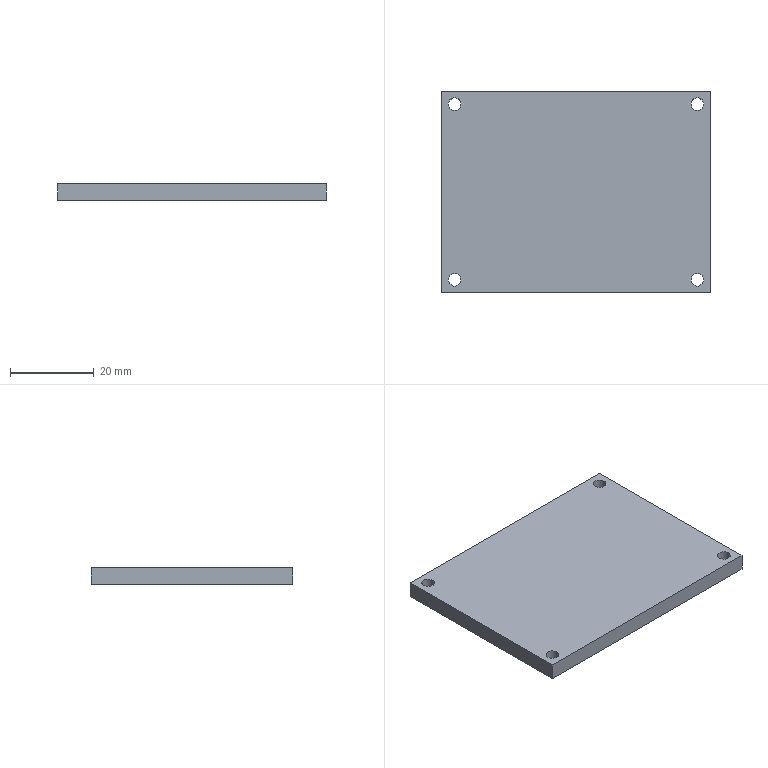Part | SolidWorks | features Extrusion 1, ICE 1 | 1 solid | 14 faces | box 64 x 48 x 4 mm | volume 12175 mm3 | cylinder 8 | plane 6 | commonest cylinder face diameters 3 x8
STEP:
#1=CARTESIAN_POINT('',(-30.45,-20.95,0.));
#2=VERTEX_POINT('',#1);
#3=CARTESIAN_POINT('',(-27.45,-20.95,0.));
#4=VERTEX_POINT('',#3);
#5=CARTESIAN_POINT('',(-28.95,-20.95,0.));
#6=DIRECTION('',(0.,0.,1.));
#7=DIRECTION('',(-1.,0.,0.));
#8=AXIS2_PLACEMENT_3D('',#5,#6,#7);
#9=CIRCLE('',#8,1.5);
#10=EDGE_CURVE('',#2,#4,#9,.T.);
#11=ORIENTED_EDGE('',*,*,#10,.F.);
#12=CARTESIAN_POINT('',(-30.45,-20.95,4.));
#13=VERTEX_POINT('',#12);
#14=CARTESIAN_POINT('',(-30.45,-20.95,0.));
#15=DIRECTION('',(0.,0.,1.));
#16=VECTOR('',#15,1000.);
#17=LINE('',#14,#16);
#18=EDGE_CURVE('',#2,#13,#17,.T.);
#19=ORIENTED_EDGE('',*,*,#18,.T.);
#20=CARTESIAN_POINT('',(-27.45,-20.95,4.));
#21=VERTEX_POINT('',#20);
#22=CARTESIAN_POINT('',(-28.95,-20.95,4.));
#23=DIRECTION('',(0.,0.,1.));
#24=DIRECTION('',(-1.,0.,0.));
#25=AXIS2_PLACEMENT_3D('',#22,#23,#24);
#26=CIRCLE('',#25,1.5);
#27=EDGE_CURVE('',#13,#21,#26,.T.);
#28=ORIENTED_EDGE('',*,*,#27,.T.);
#29=CARTESIAN_POINT('',(-27.45,-20.95,0.));
#30=DIRECTION('',(0.,0.,1.));
#31=VECTOR('',#30,1000.);
#32=LINE('',#29,#31);
#33=EDGE_CURVE('',#4,#21,#32,.T.);
#34=ORIENTED_EDGE('',*,*,#33,.F.);
#35=EDGE_LOOP('',(#11,#19,#28,#34));
#36=FACE_OUTER_BOUND('',#35,.T.);
#37=CARTESIAN_POINT('',(-28.95,-20.95,0.));
#38=DIRECTION('',(0.,0.,1.));
#39=DIRECTION('',(1.,0.,0.));
#40=AXIS2_PLACEMENT_3D('',#37,#38,#39);
#41=CYLINDRICAL_SURFACE('',#40,1.5);
#42=ADVANCED_FACE('',(#36),#41,.F.);
#43=CARTESIAN_POINT('',(27.45,20.95,0.));
#44=VERTEX_POINT('',#43);
#45=CARTESIAN_POINT('',(30.45,20.95,0.));
#46=VERTEX_POINT('',#45);
#47=CARTESIAN_POINT('',(28.95,20.95,0.));
#48=DIRECTION('',(0.,0.,1.));
#49=DIRECTION('',(-1.,0.,0.));
#50=AXIS2_PLACEMENT_3D('',#47,#48,#49);
#51=CIRCLE('',#50,1.5);
#52=EDGE_CURVE('',#44,#46,#51,.T.);
#53=ORIENTED_EDGE('',*,*,#52,.F.);
#54=CARTESIAN_POINT('',(27.45,20.95,4.));
#55=VERTEX_POINT('',#54);
#56=CARTESIAN_POINT('',(27.45,20.95,0.));
#57=DIRECTION('',(0.,0.,1.));
#58=VECTOR('',#57,1000.);
#59=LINE('',#56,#58);
#60=EDGE_CURVE('',#44,#55,#59,.T.);
#61=ORIENTED_EDGE('',*,*,#60,.T.);
#62=CARTESIAN_POINT('',(30.45,20.95,4.));
#63=VERTEX_POINT('',#62);
#64=CARTESIAN_POINT('',(28.95,20.95,4.));
#65=DIRECTION('',(0.,0.,1.));
#66=DIRECTION('',(-1.,0.,0.));
#67=AXIS2_PLACEMENT_3D('',#64,#65,#66);
#68=CIRCLE('',#67,1.5);
#69=EDGE_CURVE('',#55,#63,#68,.T.);
#70=ORIENTED_EDGE('',*,*,#69,.T.);
#71=CARTESIAN_POINT('',(30.45,20.95,0.));
#72=DIRECTION('',(0.,0.,1.));
#73=VECTOR('',#72,1000.);
#74=LINE('',#71,#73);
#75=EDGE_CURVE('',#46,#63,#74,.T.);
#76=ORIENTED_EDGE('',*,*,#75,.F.);
#77=EDGE_LOOP('',(#53,#61,#70,#76));
#78=FACE_OUTER_BOUND('',#77,.T.);
#79=CARTESIAN_POINT('',(28.95,20.95,0.));
#80=DIRECTION('',(0.,0.,1.));
#81=DIRECTION('',(1.,0.,0.));
#82=AXIS2_PLACEMENT_3D('',#79,#80,#81);
#83=CYLINDRICAL_SURFACE('',#82,1.5);
#84=ADVANCED_FACE('',(#78),#83,.F.);
#85=CARTESIAN_POINT('',(-30.45,20.95,0.));
#86=VERTEX_POINT('',#85);
#87=CARTESIAN_POINT('',(-27.45,20.95,0.));
#88=VERTEX_POINT('',#87);
#89=CARTESIAN_POINT('',(-28.95,20.95,0.));
#90=DIRECTION('',(0.,0.,1.));
#91=DIRECTION('',(1.,0.,0.));
#92=AXIS2_PLACEMENT_3D('',#89,#90,#91);
#93=CIRCLE('',#92,1.5);
#94=EDGE_CURVE('',#86,#88,#93,.T.);
#95=ORIENTED_EDGE('',*,*,#94,.F.);
#96=CARTESIAN_POINT('',(-30.45,20.95,4.));
#97=VERTEX_POINT('',#96);
#98=CARTESIAN_POINT('',(-30.45,20.95,0.));
#99=DIRECTION('',(0.,0.,1.));
#100=VECTOR('',#99,1000.);
#101=LINE('',#98,#100);
#102=EDGE_CURVE('',#86,#97,#101,.T.);
#103=ORIENTED_EDGE('',*,*,#102,.T.);
#104=CARTESIAN_POINT('',(-27.45,20.95,4.));
#105=VERTEX_POINT('',#104);
#106=CARTESIAN_POINT('',(-28.95,20.95,4.));
#107=DIRECTION('',(0.,0.,1.));
#108=DIRECTION('',(1.,0.,0.));
#109=AXIS2_PLACEMENT_3D('',#106,#107,#108);
#110=CIRCLE('',#109,1.5);
#111=EDGE_CURVE('',#97,#105,#110,.T.);
#112=ORIENTED_EDGE('',*,*,#111,.T.);
#113=CARTESIAN_POINT('',(-27.45,20.95,0.));
#114=DIRECTION('',(0.,0.,1.));
#115=VECTOR('',#114,1000.);
#116=LINE('',#113,#115);
#117=EDGE_CURVE('',#88,#105,#116,.T.);
#118=ORIENTED_EDGE('',*,*,#117,.F.);
#119=EDGE_LOOP('',(#95,#103,#112,#118));
#120=FACE_OUTER_BOUND('',#119,.T.);
#121=CARTESIAN_POINT('',(-28.95,20.95,0.));
#122=DIRECTION('',(0.,0.,1.));
#123=DIRECTION('',(1.,0.,0.));
#124=AXIS2_PLACEMENT_3D('',#121,#122,#123);
#125=CYLINDRICAL_SURFACE('',#124,1.5);
#126=ADVANCED_FACE('',(#120),#125,.F.);
#127=CARTESIAN_POINT('',(27.45,-20.95,0.));
#128=VERTEX_POINT('',#127);
#129=CARTESIAN_POINT('',(30.45,-20.95,0.));
#130=VERTEX_POINT('',#129);
#131=CARTESIAN_POINT('',(28.95,-20.95,0.));
#132=DIRECTION('',(0.,0.,1.));
#133=DIRECTION('',(1.,0.,0.));
#134=AXIS2_PLACEMENT_3D('',#131,#132,#133);
#135=CIRCLE('',#134,1.5);
#136=EDGE_CURVE('',#128,#130,#135,.T.);
#137=ORIENTED_EDGE('',*,*,#136,.F.);
#138=CARTESIAN_POINT('',(27.45,-20.95,4.));
#139=VERTEX_POINT('',#138);
#140=CARTESIAN_POINT('',(27.45,-20.95,0.));
#141=DIRECTION('',(0.,0.,1.));
#142=VECTOR('',#141,1000.);
#143=LINE('',#140,#142);
#144=EDGE_CURVE('',#128,#139,#143,.T.);
#145=ORIENTED_EDGE('',*,*,#144,.T.);
#146=CARTESIAN_POINT('',(30.45,-20.95,4.));
#147=VERTEX_POINT('',#146);
#148=CARTESIAN_POINT('',(28.95,-20.95,4.));
#149=DIRECTION('',(0.,0.,1.));
#150=DIRECTION('',(1.,0.,0.));
#151=AXIS2_PLACEMENT_3D('',#148,#149,#150);
#152=CIRCLE('',#151,1.5);
#153=EDGE_CURVE('',#139,#147,#152,.T.);
#154=ORIENTED_EDGE('',*,*,#153,.T.);
#155=CARTESIAN_POINT('',(30.45,-20.95,0.));
#156=DIRECTION('',(0.,0.,1.));
#157=VECTOR('',#156,1000.);
#158=LINE('',#155,#157);
#159=EDGE_CURVE('',#130,#147,#158,.T.);
#160=ORIENTED_EDGE('',*,*,#159,.F.);
#161=EDGE_LOOP('',(#137,#145,#154,#160));
#162=FACE_OUTER_BOUND('',#161,.T.);
#163=CARTESIAN_POINT('',(28.95,-20.95,0.));
#164=DIRECTION('',(0.,0.,1.));
#165=DIRECTION('',(1.,0.,0.));
#166=AXIS2_PLACEMENT_3D('',#163,#164,#165);
#167=CYLINDRICAL_SURFACE('',#166,1.5);
#168=ADVANCED_FACE('',(#162),#167,.F.);
#169=CARTESIAN_POINT('',(32.,-24.,0.));
#170=VERTEX_POINT('',#169);
#171=CARTESIAN_POINT('',(32.,24.,0.));
#172=VERTEX_POINT('',#171);
#173=CARTESIAN_POINT('',(32.,-24.,0.));
#174=DIRECTION('',(0.,1.,0.));
#175=VECTOR('',#174,1000.);
#176=LINE('',#173,#175);
#177=EDGE_CURVE('',#170,#172,#176,.T.);
#178=ORIENTED_EDGE('',*,*,#177,.T.);
#179=CARTESIAN_POINT('',(32.,24.,4.));
#180=VERTEX_POINT('',#179);
#181=CARTESIAN_POINT('',(32.,24.,4.));
#182=DIRECTION('',(0.,0.,-1.));
#183=VECTOR('',#182,1000.);
#184=LINE('',#181,#183);
#185=EDGE_CURVE('',#180,#172,#184,.T.);
#186=ORIENTED_EDGE('',*,*,#185,.F.);
#187=CARTESIAN_POINT('',(32.,-24.,4.));
#188=VERTEX_POINT('',#187);
#189=CARTESIAN_POINT('',(32.,-24.,4.));
#190=DIRECTION('',(0.,1.,0.));
#191=VECTOR('',#190,1000.);
#192=LINE('',#189,#191);
#193=EDGE_CURVE('',#188,#180,#192,.T.);
#194=ORIENTED_EDGE('',*,*,#193,.F.);
#195=CARTESIAN_POINT('',(32.,-24.,4.));
#196=DIRECTION('',(0.,0.,-1.));
#197=VECTOR('',#196,1000.);
#198=LINE('',#195,#197);
#199=EDGE_CURVE('',#188,#170,#198,.T.);
#200=ORIENTED_EDGE('',*,*,#199,.T.);
#201=EDGE_LOOP('',(#178,#186,#194,#200));
#202=FACE_OUTER_BOUND('',#201,.T.);
#203=CARTESIAN_POINT('',(32.,-24.,4.));
#204=DIRECTION('',(-1.,0.,0.));
#205=DIRECTION('',(0.,0.,1.));
#206=AXIS2_PLACEMENT_3D('',#203,#204,#205);
#207=PLANE('',#206);
#208=ADVANCED_FACE('',(#202),#207,.F.);
#209=CARTESIAN_POINT('',(-32.,24.,0.));
#210=VERTEX_POINT('',#209);
#211=CARTESIAN_POINT('',(-32.,24.,0.));
#212=DIRECTION('',(-1.,0.,0.));
#213=VECTOR('',#212,1000.);
#214=LINE('',#211,#213);
#215=EDGE_CURVE('',#172,#210,#214,.T.);
#216=ORIENTED_EDGE('',*,*,#215,.T.);
#217=CARTESIAN_POINT('',(-32.,24.,4.));
#218=VERTEX_POINT('',#217);
#219=CARTESIAN_POINT('',(-32.,24.,4.));
#220=DIRECTION('',(0.,0.,-1.));
#221=VECTOR('',#220,1000.);
#222=LINE('',#219,#221);
#223=EDGE_CURVE('',#218,#210,#222,.T.);
#224=ORIENTED_EDGE('',*,*,#223,.F.);
#225=CARTESIAN_POINT('',(-32.,24.,4.));
#226=DIRECTION('',(-1.,0.,0.));
#227=VECTOR('',#226,1000.);
#228=LINE('',#225,#227);
#229=EDGE_CURVE('',#180,#218,#228,.T.);
#230=ORIENTED_EDGE('',*,*,#229,.F.);
#231=ORIENTED_EDGE('',*,*,#185,.T.);
#232=EDGE_LOOP('',(#216,#224,#230,#231));
#233=FACE_OUTER_BOUND('',#232,.T.);
#234=CARTESIAN_POINT('',(-32.,24.,4.));
#235=DIRECTION('',(0.,-1.,0.));
#236=DIRECTION('',(0.,0.,-1.));
#237=AXIS2_PLACEMENT_3D('',#234,#235,#236);
#238=PLANE('',#237);
#239=ADVANCED_FACE('',(#233),#238,.F.);
#240=CARTESIAN_POINT('',(-32.,-24.,0.));
#241=VERTEX_POINT('',#240);
#242=CARTESIAN_POINT('',(-32.,-24.,0.));
#243=DIRECTION('',(0.,-1.,0.));
#244=VECTOR('',#243,1000.);
#245=LINE('',#242,#244);
#246=EDGE_CURVE('',#210,#241,#245,.T.);
#247=ORIENTED_EDGE('',*,*,#246,.T.);
#248=CARTESIAN_POINT('',(-32.,-24.,4.));
#249=VERTEX_POINT('',#248);
#250=CARTESIAN_POINT('',(-32.,-24.,4.));
#251=DIRECTION('',(0.,0.,-1.));
#252=VECTOR('',#251,1000.);
#253=LINE('',#250,#252);
#254=EDGE_CURVE('',#249,#241,#253,.T.);
#255=ORIENTED_EDGE('',*,*,#254,.F.);
#256=CARTESIAN_POINT('',(-32.,-24.,4.));
#257=DIRECTION('',(0.,-1.,0.));
#258=VECTOR('',#257,1000.);
#259=LINE('',#256,#258);
#260=EDGE_CURVE('',#218,#249,#259,.T.);
#261=ORIENTED_EDGE('',*,*,#260,.F.);
#262=ORIENTED_EDGE('',*,*,#223,.T.);
#263=EDGE_LOOP('',(#247,#255,#261,#262));
#264=FACE_OUTER_BOUND('',#263,.T.);
#265=CARTESIAN_POINT('',(-32.,-24.,4.));
#266=DIRECTION('',(1.,0.,0.));
#267=DIRECTION('',(0.,0.,-1.));
#268=AXIS2_PLACEMENT_3D('',#265,#266,#267);
#269=PLANE('',#268);
#270=ADVANCED_FACE('',(#264),#269,.F.);
#271=CARTESIAN_POINT('',(-32.,-24.,0.));
#272=DIRECTION('',(1.,0.,0.));
#273=VECTOR('',#272,1000.);
#274=LINE('',#271,#273);
#275=EDGE_CURVE('',#241,#170,#274,.T.);
#276=ORIENTED_EDGE('',*,*,#275,.T.);
#277=ORIENTED_EDGE('',*,*,#199,.F.);
#278=CARTESIAN_POINT('',(-32.,-24.,4.));
#279=DIRECTION('',(1.,0.,0.));
#280=VECTOR('',#279,1000.);
#281=LINE('',#278,#280);
#282=EDGE_CURVE('',#249,#188,#281,.T.);
#283=ORIENTED_EDGE('',*,*,#282,.F.);
#284=ORIENTED_EDGE('',*,*,#254,.T.);
#285=EDGE_LOOP('',(#276,#277,#283,#284));
#286=FACE_OUTER_BOUND('',#285,.T.);
#287=CARTESIAN_POINT('',(-32.,-24.,4.));
#288=DIRECTION('',(0.,1.,0.));
#289=DIRECTION('',(0.,0.,1.));
#290=AXIS2_PLACEMENT_3D('',#287,#288,#289);
#291=PLANE('',#290);
#292=ADVANCED_FACE('',(#286),#291,.F.);
#293=CARTESIAN_POINT('',(-28.95,-20.95,4.));
#294=DIRECTION('',(0.,0.,1.));
#295=DIRECTION('',(-1.,0.,0.));
#296=AXIS2_PLACEMENT_3D('',#293,#294,#295);
#297=CIRCLE('',#296,1.5);
#298=EDGE_CURVE('',#21,#13,#297,.T.);
#299=ORIENTED_EDGE('',*,*,#298,.F.);
#300=ORIENTED_EDGE('',*,*,#27,.F.);
#301=EDGE_LOOP('',(#299,#300));
#302=FACE_BOUND('',#301,.T.);
#303=CARTESIAN_POINT('',(28.95,20.95,4.));
#304=DIRECTION('',(0.,0.,1.));
#305=DIRECTION('',(-1.,0.,0.));
#306=AXIS2_PLACEMENT_3D('',#303,#304,#305);
#307=CIRCLE('',#306,1.5);
#308=EDGE_CURVE('',#63,#55,#307,.T.);
#309=ORIENTED_EDGE('',*,*,#308,.F.);
#310=ORIENTED_EDGE('',*,*,#69,.F.);
#311=EDGE_LOOP('',(#309,#310));
#312=FACE_BOUND('',#311,.T.);
#313=CARTESIAN_POINT('',(-28.95,20.95,4.));
#314=DIRECTION('',(0.,0.,1.));
#315=DIRECTION('',(1.,0.,0.));
#316=AXIS2_PLACEMENT_3D('',#313,#314,#315);
#317=CIRCLE('',#316,1.5);
#318=EDGE_CURVE('',#105,#97,#317,.T.);
#319=ORIENTED_EDGE('',*,*,#318,.F.);
#320=ORIENTED_EDGE('',*,*,#111,.F.);
#321=EDGE_LOOP('',(#319,#320));
#322=FACE_BOUND('',#321,.T.);
#323=CARTESIAN_POINT('',(28.95,-20.95,4.));
#324=DIRECTION('',(0.,0.,1.));
#325=DIRECTION('',(1.,0.,0.));
#326=AXIS2_PLACEMENT_3D('',#323,#324,#325);
#327=CIRCLE('',#326,1.5);
#328=EDGE_CURVE('',#147,#139,#327,.T.);
#329=ORIENTED_EDGE('',*,*,#328,.F.);
#330=ORIENTED_EDGE('',*,*,#153,.F.);
#331=EDGE_LOOP('',(#329,#330));
#332=FACE_BOUND('',#331,.T.);
#333=ORIENTED_EDGE('',*,*,#193,.T.);
#334=ORIENTED_EDGE('',*,*,#229,.T.);
#335=ORIENTED_EDGE('',*,*,#260,.T.);
#336=ORIENTED_EDGE('',*,*,#282,.T.);
#337=EDGE_LOOP('',(#333,#334,#335,#336));
#338=FACE_OUTER_BOUND('',#337,.T.);
#339=CARTESIAN_POINT('',(0.,0.,4.));
#340=DIRECTION('',(0.,0.,-1.));
#341=DIRECTION('',(-1.,0.,0.));
#342=AXIS2_PLACEMENT_3D('',#339,#340,#341);
#343=PLANE('',#342);
#344=ADVANCED_FACE('',(#302,#312,#322,#332,#338),#343,.F.);
#345=CARTESIAN_POINT('',(-28.95,-20.95,0.));
#346=DIRECTION('',(0.,0.,1.));
#347=DIRECTION('',(-1.,0.,0.));
#348=AXIS2_PLACEMENT_3D('',#345,#346,#347);
#349=CIRCLE('',#348,1.5);
#350=EDGE_CURVE('',#4,#2,#349,.T.);
#351=ORIENTED_EDGE('',*,*,#350,.T.);
#352=ORIENTED_EDGE('',*,*,#10,.T.);
#353=EDGE_LOOP('',(#351,#352));
#354=FACE_BOUND('',#353,.T.);
#355=CARTESIAN_POINT('',(28.95,20.95,0.));
#356=DIRECTION('',(0.,0.,1.));
#357=DIRECTION('',(-1.,0.,0.));
#358=AXIS2_PLACEMENT_3D('',#355,#356,#357);
#359=CIRCLE('',#358,1.5);
#360=EDGE_CURVE('',#46,#44,#359,.T.);
#361=ORIENTED_EDGE('',*,*,#360,.T.);
#362=ORIENTED_EDGE('',*,*,#52,.T.);
#363=EDGE_LOOP('',(#361,#362));
#364=FACE_BOUND('',#363,.T.);
#365=CARTESIAN_POINT('',(-28.95,20.95,0.));
#366=DIRECTION('',(0.,0.,1.));
#367=DIRECTION('',(1.,0.,0.));
#368=AXIS2_PLACEMENT_3D('',#365,#366,#367);
#369=CIRCLE('',#368,1.5);
#370=EDGE_CURVE('',#88,#86,#369,.T.);
#371=ORIENTED_EDGE('',*,*,#370,.T.);
#372=ORIENTED_EDGE('',*,*,#94,.T.);
#373=EDGE_LOOP('',(#371,#372));
#374=FACE_BOUND('',#373,.T.);
#375=CARTESIAN_POINT('',(28.95,-20.95,0.));
#376=DIRECTION('',(0.,0.,1.));
#377=DIRECTION('',(1.,0.,0.));
#378=AXIS2_PLACEMENT_3D('',#375,#376,#377);
#379=CIRCLE('',#378,1.5);
#380=EDGE_CURVE('',#130,#128,#379,.T.);
#381=ORIENTED_EDGE('',*,*,#380,.T.);
#382=ORIENTED_EDGE('',*,*,#136,.T.);
#383=EDGE_LOOP('',(#381,#382));
#384=FACE_BOUND('',#383,.T.);
#385=ORIENTED_EDGE('',*,*,#177,.F.);
#386=ORIENTED_EDGE('',*,*,#275,.F.);
#387=ORIENTED_EDGE('',*,*,#246,.F.);
#388=ORIENTED_EDGE('',*,*,#215,.F.);
#389=EDGE_LOOP('',(#385,#386,#387,#388));
#390=FACE_OUTER_BOUND('',#389,.T.);
#391=CARTESIAN_POINT('',(0.,0.,0.));
#392=DIRECTION('',(0.,0.,-1.));
#393=DIRECTION('',(-1.,0.,0.));
#394=AXIS2_PLACEMENT_3D('',#391,#392,#393);
#395=PLANE('',#394);
#396=ADVANCED_FACE('',(#354,#364,#374,#384,#390),#395,.T.);
#397=ORIENTED_EDGE('',*,*,#144,.F.);
#398=ORIENTED_EDGE('',*,*,#380,.F.);
#399=ORIENTED_EDGE('',*,*,#159,.T.);
#400=ORIENTED_EDGE('',*,*,#328,.T.);
#401=EDGE_LOOP('',(#397,#398,#399,#400));
#402=FACE_OUTER_BOUND('',#401,.T.);
#403=CARTESIAN_POINT('',(28.95,-20.95,0.));
#404=DIRECTION('',(0.,0.,1.));
#405=DIRECTION('',(1.,0.,0.));
#406=AXIS2_PLACEMENT_3D('',#403,#404,#405);
#407=CYLINDRICAL_SURFACE('',#406,1.5);
#408=ADVANCED_FACE('',(#402),#407,.F.);
#409=ORIENTED_EDGE('',*,*,#102,.F.);
#410=ORIENTED_EDGE('',*,*,#370,.F.);
#411=ORIENTED_EDGE('',*,*,#117,.T.);
#412=ORIENTED_EDGE('',*,*,#318,.T.);
#413=EDGE_LOOP('',(#409,#410,#411,#412));
#414=FACE_OUTER_BOUND('',#413,.T.);
#415=CARTESIAN_POINT('',(-28.95,20.95,0.));
#416=DIRECTION('',(0.,0.,1.));
#417=DIRECTION('',(1.,0.,0.));
#418=AXIS2_PLACEMENT_3D('',#415,#416,#417);
#419=CYLINDRICAL_SURFACE('',#418,1.5);
#420=ADVANCED_FACE('',(#414),#419,.F.);
#421=ORIENTED_EDGE('',*,*,#60,.F.);
#422=ORIENTED_EDGE('',*,*,#360,.F.);
#423=ORIENTED_EDGE('',*,*,#75,.T.);
#424=ORIENTED_EDGE('',*,*,#308,.T.);
#425=EDGE_LOOP('',(#421,#422,#423,#424));
#426=FACE_OUTER_BOUND('',#425,.T.);
#427=CARTESIAN_POINT('',(28.95,20.95,0.));
#428=DIRECTION('',(0.,0.,1.));
#429=DIRECTION('',(1.,0.,0.));
#430=AXIS2_PLACEMENT_3D('',#427,#428,#429);
#431=CYLINDRICAL_SURFACE('',#430,1.5);
#432=ADVANCED_FACE('',(#426),#431,.F.);
#433=ORIENTED_EDGE('',*,*,#18,.F.);
#434=ORIENTED_EDGE('',*,*,#350,.F.);
#435=ORIENTED_EDGE('',*,*,#33,.T.);
#436=ORIENTED_EDGE('',*,*,#298,.T.);
#437=EDGE_LOOP('',(#433,#434,#435,#436));
#438=FACE_OUTER_BOUND('',#437,.T.);
#439=CARTESIAN_POINT('',(-28.95,-20.95,0.));
#440=DIRECTION('',(0.,0.,1.));
#441=DIRECTION('',(1.,0.,0.));
#442=AXIS2_PLACEMENT_3D('',#439,#440,#441);
#443=CYLINDRICAL_SURFACE('',#442,1.5);
#444=ADVANCED_FACE('',(#438),#443,.F.);
#445=CLOSED_SHELL('',(#42,#84,#126,#168,#208,#239,#270,#292,#344,#396,#408,#420,#432,#444));
#446=MANIFOLD_SOLID_BREP('',#445);
#447=CARTESIAN_POINT('',(0.,0.,0.));
#448=DIRECTION('',(0.,0.,1.));
#449=DIRECTION('',(1.,0.,0.));
#450=AXIS2_PLACEMENT_3D('',#447,#448,#449);
#451=(LENGTH_UNIT()NAMED_UNIT(*)SI_UNIT(.MILLI.,.METRE.));
#452=UNCERTAINTY_MEASURE_WITH_UNIT(LENGTH_MEASURE(0.00001),#451,'','');
#453=(NAMED_UNIT(*)PLANE_ANGLE_UNIT()SI_UNIT($,.RADIAN.));
#454=(NAMED_UNIT(*)SI_UNIT($,.STERADIAN.)SOLID_ANGLE_UNIT());
#455=(GEOMETRIC_REPRESENTATION_CONTEXT(3)GLOBAL_UNCERTAINTY_ASSIGNED_CONTEXT((#452))GLOBAL_UNIT_ASSIGNED_CONTEXT((#451,#453,#454))REPRESENTATION_CONTEXT('',''));
#456=ADVANCED_BREP_SHAPE_REPRESENTATION('',(#446,#450),#455);